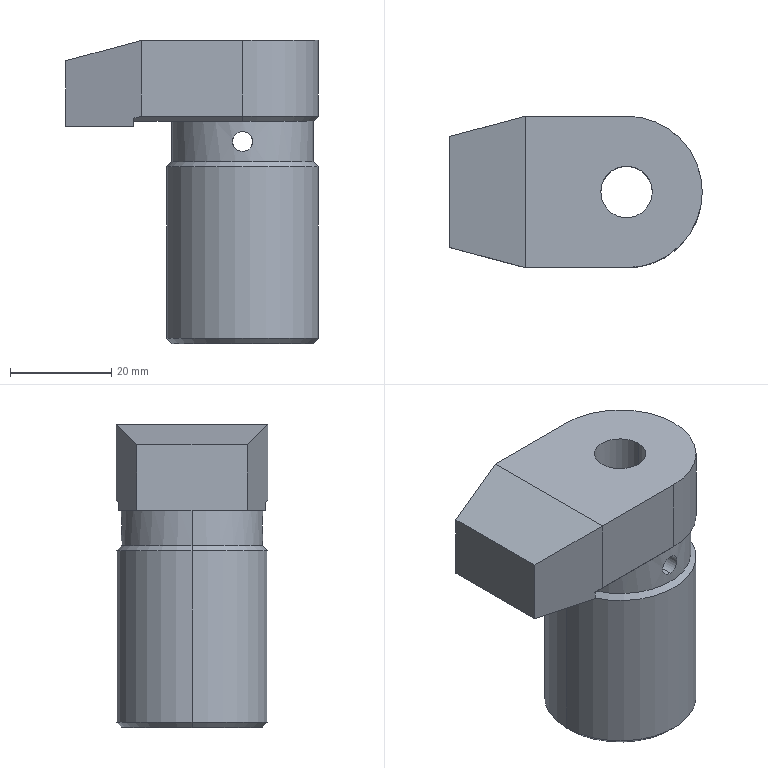Part | SolidWorks | features ICE 7, Chamfer 2, 3DProfileFeature 1, Extrusion 1, HoleWzd 1, MirrorPattern 1 | 1 solid | 36 faces | box 50 x 30 x 60 mm | volume 40900 mm3 | cylinder 15 | plane 13 | cone 8 | commonest cylinder face diameters 4 x4 30 x4 10.2 x2 18 x2 28 x2 52 x1
STEP:
#1=CARTESIAN_POINT('',(0.,14.,-22.));
#2=VERTEX_POINT('',#1);
#3=CARTESIAN_POINT('',(0.,14.,-18.));
#4=VERTEX_POINT('',#3);
#5=CARTESIAN_POINT('',(0.,14.,-22.));
#6=CARTESIAN_POINT('',(-0.1323,14.,-22.));
#7=CARTESIAN_POINT('',(-0.2624,13.998,-21.987));
#8=CARTESIAN_POINT('',(-0.5183,13.991,-21.936));
#9=CARTESIAN_POINT('',(-0.6454,13.986,-21.898));
#10=CARTESIAN_POINT('',(-0.8875,13.972,-21.797));
#11=CARTESIAN_POINT('',(-1.002,13.964,-21.736));
#12=CARTESIAN_POINT('',(-1.22,13.947,-21.59));
#13=CARTESIAN_POINT('',(-1.322,13.938,-21.506));
#14=CARTESIAN_POINT('',(-1.599,13.91,-21.23));
#15=CARTESIAN_POINT('',(-1.748,13.891,-21.007));
#16=CARTESIAN_POINT('',(-1.947,13.864,-20.525));
#17=CARTESIAN_POINT('',(-2.,13.856,-20.262));
#18=CARTESIAN_POINT('',(-2.,13.856,-19.87));
#19=CARTESIAN_POINT('',(-1.987,13.858,-19.737));
#20=CARTESIAN_POINT('',(-1.936,13.866,-19.481));
#21=CARTESIAN_POINT('',(-1.898,13.871,-19.356));
#22=CARTESIAN_POINT('',(-1.798,13.884,-19.114));
#23=CARTESIAN_POINT('',(-1.735,13.892,-18.997));
#24=CARTESIAN_POINT('',(-1.59,13.91,-18.78));
#25=CARTESIAN_POINT('',(-1.508,13.919,-18.679));
#26=CARTESIAN_POINT('',(-1.321,13.938,-18.493));
#27=CARTESIAN_POINT('',(-1.22,13.947,-18.41));
#28=CARTESIAN_POINT('',(-1.004,13.964,-18.265));
#29=CARTESIAN_POINT('',(-0.8867,13.972,-18.203));
#30=CARTESIAN_POINT('',(-0.6447,13.986,-18.102));
#31=CARTESIAN_POINT('',(-0.52,13.991,-18.064));
#32=CARTESIAN_POINT('',(-0.2633,13.998,-18.013));
#33=CARTESIAN_POINT('',(-0.1306,14.,-18.));
#34=CARTESIAN_POINT('',(0.,14.,-18.));
#35=B_SPLINE_CURVE_WITH_KNOTS('',3,(#5,#6,#7,#8,#9,#10,#11,#12,#13,#14,#15,#16,#17,#18,#19,#20,#21,#22,#23,#24,#25,#26,#27,#28,#29,#30,#31,#32,#33,#34),.UNSPECIFIED.,.F.,.F.,(4,2,2,2,2,2,2,2,2,2,2,2,2,2,4),(0.,0.0003913,0.0007826,0.001174,0.001565,0.002348,0.00313,0.003522,0.003913,0.004304,0.004696,0.005087,0.005478,0.00587,0.006261),.UNSPECIFIED.);
#36=EDGE_CURVE('',#2,#4,#35,.T.);
#37=ORIENTED_EDGE('',*,*,#36,.T.);
#38=CARTESIAN_POINT('',(0.,5.1,-18.));
#39=VERTEX_POINT('',#38);
#40=CARTESIAN_POINT('',(0.,30.,-18.));
#41=DIRECTION('',(0.,-1.,0.));
#42=VECTOR('',#41,1000.);
#43=LINE('',#40,#42);
#44=EDGE_CURVE('',#4,#39,#43,.T.);
#45=ORIENTED_EDGE('',*,*,#44,.T.);
#46=CARTESIAN_POINT('',(0.,5.1,-22.));
#47=VERTEX_POINT('',#46);
#48=CARTESIAN_POINT('',(0.,5.1,-18.));
#49=CARTESIAN_POINT('',(-0.1316,5.1,-18.));
#50=CARTESIAN_POINT('',(-0.2648,5.095,-18.013));
#51=CARTESIAN_POINT('',(-0.5241,5.075,-18.065));
#52=CARTESIAN_POINT('',(-0.6493,5.06,-18.104));
#53=CARTESIAN_POINT('',(-0.8913,5.023,-18.205));
#54=CARTESIAN_POINT('',(-1.008,5.001,-18.268));
#55=CARTESIAN_POINT('',(-1.223,4.952,-18.412));
#56=CARTESIAN_POINT('',(-1.323,4.926,-18.495));
#57=CARTESIAN_POINT('',(-1.508,4.873,-18.68));
#58=CARTESIAN_POINT('',(-1.59,4.846,-18.78));
#59=CARTESIAN_POINT('',(-1.734,4.797,-18.995));
#60=CARTESIAN_POINT('',(-1.796,4.773,-19.111));
#61=CARTESIAN_POINT('',(-1.897,4.734,-19.353));
#62=CARTESIAN_POINT('',(-1.935,4.719,-19.478));
#63=CARTESIAN_POINT('',(-1.987,4.697,-19.735));
#64=CARTESIAN_POINT('',(-2.,4.691,-19.869));
#65=CARTESIAN_POINT('',(-2.,4.692,-20.265));
#66=CARTESIAN_POINT('',(-1.946,4.715,-20.53));
#67=CARTESIAN_POINT('',(-1.795,4.774,-20.891));
#68=CARTESIAN_POINT('',(-1.732,4.797,-21.008));
#69=CARTESIAN_POINT('',(-1.587,4.847,-21.224));
#70=CARTESIAN_POINT('',(-1.505,4.874,-21.323));
#71=CARTESIAN_POINT('',(-1.322,4.927,-21.507));
#72=CARTESIAN_POINT('',(-1.22,4.953,-21.59));
#73=CARTESIAN_POINT('',(-1.005,5.001,-21.734));
#74=CARTESIAN_POINT('',(-0.8903,5.023,-21.796));
#75=CARTESIAN_POINT('',(-0.5249,5.079,-21.948));
#76=CARTESIAN_POINT('',(-0.2671,5.1,-22.));
#77=CARTESIAN_POINT('',(0.,5.1,-22.));
#78=B_SPLINE_CURVE_WITH_KNOTS('',3,(#48,#49,#50,#51,#52,#53,#54,#55,#56,#57,#58,#59,#60,#61,#62,#63,#64,#65,#66,#67,#68,#69,#70,#71,#72,#73,#74,#75,#76,#77),.UNSPECIFIED.,.F.,.F.,(4,2,2,2,2,2,2,2,2,2,2,2,2,2,4),(0.006317,0.006712,0.007106,0.007501,0.007896,0.008291,0.008685,0.00908,0.009475,0.01026,0.01066,0.01105,0.01145,0.01184,0.01263),.UNSPECIFIED.);
#79=EDGE_CURVE('',#39,#47,#78,.T.);
#80=ORIENTED_EDGE('',*,*,#79,.T.);
#81=CARTESIAN_POINT('',(0.,30.,-22.));
#82=DIRECTION('',(0.,-1.,0.));
#83=VECTOR('',#82,1000.);
#84=LINE('',#81,#83);
#85=EDGE_CURVE('',#2,#47,#84,.T.);
#86=ORIENTED_EDGE('',*,*,#85,.F.);
#87=EDGE_LOOP('',(#37,#45,#80,#86));
#88=FACE_OUTER_BOUND('',#87,.T.);
#89=CARTESIAN_POINT('',(0.,30.,-20.));
#90=DIRECTION('',(0.,-1.,0.));
#91=DIRECTION('',(0.,0.,-1.));
#92=AXIS2_PLACEMENT_3D('',#89,#90,#91);
#93=CYLINDRICAL_SURFACE('',#92,2.);
#94=ADVANCED_FACE('',(#88),#93,.F.);
#95=CARTESIAN_POINT('',(0.,-5.1,-22.));
#96=VERTEX_POINT('',#95);
#97=CARTESIAN_POINT('',(0.,-5.1,-18.));
#98=VERTEX_POINT('',#97);
#99=CARTESIAN_POINT('',(0.,-5.1,-22.));
#100=CARTESIAN_POINT('',(-0.1336,-5.1,-22.));
#101=CARTESIAN_POINT('',(-0.2647,-5.095,-21.987));
#102=CARTESIAN_POINT('',(-0.5222,-5.075,-21.935));
#103=CARTESIAN_POINT('',(-0.65,-5.06,-21.896));
#104=CARTESIAN_POINT('',(-0.8917,-5.023,-21.795));
#105=CARTESIAN_POINT('',(-1.006,-5.001,-21.733));
#106=CARTESIAN_POINT('',(-1.223,-4.953,-21.588));
#107=CARTESIAN_POINT('',(-1.324,-4.926,-21.505));
#108=CARTESIAN_POINT('',(-1.598,-4.847,-21.231));
#109=CARTESIAN_POINT('',(-1.746,-4.793,-21.01));
#110=CARTESIAN_POINT('',(-1.896,-4.735,-20.65));
#111=CARTESIAN_POINT('',(-1.935,-4.719,-20.523));
#112=CARTESIAN_POINT('',(-1.987,-4.697,-20.264));
#113=CARTESIAN_POINT('',(-2.,-4.692,-20.133));
#114=CARTESIAN_POINT('',(-2.,-4.691,-19.869));
#115=CARTESIAN_POINT('',(-1.987,-4.697,-19.735));
#116=CARTESIAN_POINT('',(-1.935,-4.719,-19.477));
#117=CARTESIAN_POINT('',(-1.897,-4.734,-19.352));
#118=CARTESIAN_POINT('',(-1.795,-4.774,-19.108));
#119=CARTESIAN_POINT('',(-1.733,-4.797,-18.994));
#120=CARTESIAN_POINT('',(-1.589,-4.847,-18.778));
#121=CARTESIAN_POINT('',(-1.505,-4.874,-18.677));
#122=CARTESIAN_POINT('',(-1.322,-4.927,-18.494));
#123=CARTESIAN_POINT('',(-1.222,-4.953,-18.412));
#124=CARTESIAN_POINT('',(-1.006,-5.001,-18.267));
#125=CARTESIAN_POINT('',(-0.8896,-5.023,-18.204));
#126=CARTESIAN_POINT('',(-0.5289,-5.078,-18.054));
#127=CARTESIAN_POINT('',(-0.2632,-5.1,-18.));
#128=CARTESIAN_POINT('',(0.,-5.1,-18.));
#129=B_SPLINE_CURVE_WITH_KNOTS('',3,(#99,#100,#101,#102,#103,#104,#105,#106,#107,#108,#109,#110,#111,#112,#113,#114,#115,#116,#117,#118,#119,#120,#121,#122,#123,#124,#125,#126,#127,#128),.UNSPECIFIED.,.F.,.F.,(4,2,2,2,2,2,2,2,2,2,2,2,2,2,4),(0.,0.0003948,0.0007896,0.001184,0.001579,0.002369,0.002764,0.003158,0.003553,0.003948,0.004343,0.004738,0.005133,0.005527,0.006317),.UNSPECIFIED.);
#130=EDGE_CURVE('',#96,#98,#129,.T.);
#131=ORIENTED_EDGE('',*,*,#130,.T.);
#132=CARTESIAN_POINT('',(0.,-14.,-18.));
#133=VERTEX_POINT('',#132);
#134=CARTESIAN_POINT('',(0.,30.,-18.));
#135=DIRECTION('',(0.,-1.,0.));
#136=VECTOR('',#135,1000.);
#137=LINE('',#134,#136);
#138=EDGE_CURVE('',#98,#133,#137,.T.);
#139=ORIENTED_EDGE('',*,*,#138,.T.);
#140=CARTESIAN_POINT('',(0.,-14.,-22.));
#141=VERTEX_POINT('',#140);
#142=CARTESIAN_POINT('',(0.,-14.,-18.));
#143=CARTESIAN_POINT('',(-0.2612,-14.,-18.));
#144=CARTESIAN_POINT('',(-0.5246,-13.992,-18.053));
#145=CARTESIAN_POINT('',(-1.006,-13.966,-18.252));
#146=CARTESIAN_POINT('',(-1.229,-13.947,-18.401));
#147=CARTESIAN_POINT('',(-1.506,-13.919,-18.677));
#148=CARTESIAN_POINT('',(-1.59,-13.91,-18.78));
#149=CARTESIAN_POINT('',(-1.735,-13.892,-18.997));
#150=CARTESIAN_POINT('',(-1.797,-13.884,-19.111));
#151=CARTESIAN_POINT('',(-1.897,-13.871,-19.354));
#152=CARTESIAN_POINT('',(-1.936,-13.866,-19.481));
#153=CARTESIAN_POINT('',(-1.987,-13.858,-19.736));
#154=CARTESIAN_POINT('',(-2.,-13.856,-19.866));
#155=CARTESIAN_POINT('',(-2.,-13.856,-20.131));
#156=CARTESIAN_POINT('',(-1.987,-13.858,-20.261));
#157=CARTESIAN_POINT('',(-1.936,-13.865,-20.517));
#158=CARTESIAN_POINT('',(-1.898,-13.871,-20.644));
#159=CARTESIAN_POINT('',(-1.798,-13.884,-20.886));
#160=CARTESIAN_POINT('',(-1.736,-13.892,-21.001));
#161=CARTESIAN_POINT('',(-1.591,-13.909,-21.218));
#162=CARTESIAN_POINT('',(-1.507,-13.919,-21.321));
#163=CARTESIAN_POINT('',(-1.231,-13.947,-21.598));
#164=CARTESIAN_POINT('',(-1.008,-13.966,-21.747));
#165=CARTESIAN_POINT('',(-0.5274,-13.992,-21.947));
#166=CARTESIAN_POINT('',(-0.2646,-14.,-22.));
#167=CARTESIAN_POINT('',(0.,-14.,-22.));
#168=B_SPLINE_CURVE_WITH_KNOTS('',3,(#142,#143,#144,#145,#146,#147,#148,#149,#150,#151,#152,#153,#154,#155,#156,#157,#158,#159,#160,#161,#162,#163,#164,#165,#166,#167),.UNSPECIFIED.,.F.,.F.,(4,2,2,2,2,2,2,2,2,2,2,2,4),(0.006261,0.007043,0.007826,0.008217,0.008608,0.008999,0.009391,0.009782,0.01017,0.01056,0.01096,0.01174,0.01252),.UNSPECIFIED.);
#169=EDGE_CURVE('',#133,#141,#168,.T.);
#170=ORIENTED_EDGE('',*,*,#169,.T.);
#171=CARTESIAN_POINT('',(0.,30.,-22.));
#172=DIRECTION('',(0.,-1.,0.));
#173=VECTOR('',#172,1000.);
#174=LINE('',#171,#173);
#175=EDGE_CURVE('',#96,#141,#174,.T.);
#176=ORIENTED_EDGE('',*,*,#175,.F.);
#177=EDGE_LOOP('',(#131,#139,#170,#176));
#178=FACE_OUTER_BOUND('',#177,.T.);
#179=CARTESIAN_POINT('',(0.,30.,-20.));
#180=DIRECTION('',(0.,-1.,0.));
#181=DIRECTION('',(0.,0.,-1.));
#182=AXIS2_PLACEMENT_3D('',#179,#180,#181);
#183=CYLINDRICAL_SURFACE('',#182,2.);
#184=ADVANCED_FACE('',(#178),#183,.F.);
#185=CARTESIAN_POINT('',(9.,0.,-59.));
#186=VERTEX_POINT('',#185);
#187=CARTESIAN_POINT('',(-9.,0.,-59.));
#188=VERTEX_POINT('',#187);
#189=CARTESIAN_POINT('',(0.,0.,-59.));
#190=DIRECTION('',(0.,0.,-1.));
#191=DIRECTION('',(-1.,0.,0.));
#192=AXIS2_PLACEMENT_3D('',#189,#190,#191);
#193=CIRCLE('',#192,9.);
#194=EDGE_CURVE('',#186,#188,#193,.T.);
#195=ORIENTED_EDGE('',*,*,#194,.F.);
#196=CARTESIAN_POINT('',(10.,0.,-60.));
#197=VERTEX_POINT('',#196);
#198=CARTESIAN_POINT('',(9.,0.,-59.));
#199=DIRECTION('',(0.7071,0.,-0.7071));
#200=VECTOR('',#199,1000.);
#201=LINE('',#198,#200);
#202=EDGE_CURVE('',#186,#197,#201,.T.);
#203=ORIENTED_EDGE('',*,*,#202,.T.);
#204=CARTESIAN_POINT('',(-10.,0.,-60.));
#205=VERTEX_POINT('',#204);
#206=CARTESIAN_POINT('',(0.,0.,-60.));
#207=DIRECTION('',(0.,0.,1.));
#208=DIRECTION('',(-1.,0.,0.));
#209=AXIS2_PLACEMENT_3D('',#206,#207,#208);
#210=CIRCLE('',#209,10.);
#211=EDGE_CURVE('',#205,#197,#210,.T.);
#212=ORIENTED_EDGE('',*,*,#211,.F.);
#213=CARTESIAN_POINT('',(-9.,0.,-59.));
#214=DIRECTION('',(-0.7071,0.,-0.7071));
#215=VECTOR('',#214,1000.);
#216=LINE('',#213,#215);
#217=EDGE_CURVE('',#188,#205,#216,.T.);
#218=ORIENTED_EDGE('',*,*,#217,.F.);
#219=EDGE_LOOP('',(#195,#203,#212,#218));
#220=FACE_OUTER_BOUND('',#219,.T.);
#221=CARTESIAN_POINT('',(0.,0.,-59.));
#222=DIRECTION('',(0.,0.,-1.));
#223=DIRECTION('',(-1.,0.,0.));
#224=AXIS2_PLACEMENT_3D('',#221,#222,#223);
#225=CONICAL_SURFACE('',#224,9.,0.7854);
#226=ADVANCED_FACE('',(#220),#225,.F.);
#227=CARTESIAN_POINT('',(-14.,0.,-60.));
#228=VERTEX_POINT('',#227);
#229=CARTESIAN_POINT('',(14.,0.,-60.));
#230=VERTEX_POINT('',#229);
#231=CARTESIAN_POINT('',(0.,0.,-60.));
#232=DIRECTION('',(0.,0.,-1.));
#233=DIRECTION('',(-1.,0.,0.));
#234=AXIS2_PLACEMENT_3D('',#231,#232,#233);
#235=CIRCLE('',#234,14.);
#236=EDGE_CURVE('',#228,#230,#235,.T.);
#237=ORIENTED_EDGE('',*,*,#236,.F.);
#238=CARTESIAN_POINT('',(-15.,0.,-59.));
#239=VERTEX_POINT('',#238);
#240=CARTESIAN_POINT('',(-14.,0.,-60.));
#241=DIRECTION('',(-0.7071,0.,0.7071));
#242=VECTOR('',#241,1000.);
#243=LINE('',#240,#242);
#244=EDGE_CURVE('',#228,#239,#243,.T.);
#245=ORIENTED_EDGE('',*,*,#244,.T.);
#246=CARTESIAN_POINT('',(15.,0.,-59.));
#247=VERTEX_POINT('',#246);
#248=CARTESIAN_POINT('',(0.,0.,-59.));
#249=DIRECTION('',(0.,0.,1.));
#250=DIRECTION('',(-1.,0.,0.));
#251=AXIS2_PLACEMENT_3D('',#248,#249,#250);
#252=CIRCLE('',#251,15.);
#253=EDGE_CURVE('',#247,#239,#252,.T.);
#254=ORIENTED_EDGE('',*,*,#253,.F.);
#255=CARTESIAN_POINT('',(14.,0.,-60.));
#256=DIRECTION('',(0.7071,0.,0.7071));
#257=VECTOR('',#256,1000.);
#258=LINE('',#255,#257);
#259=EDGE_CURVE('',#230,#247,#258,.T.);
#260=ORIENTED_EDGE('',*,*,#259,.F.);
#261=EDGE_LOOP('',(#237,#245,#254,#260));
#262=FACE_OUTER_BOUND('',#261,.T.);
#263=CARTESIAN_POINT('',(0.,0.,-60.));
#264=DIRECTION('',(0.,0.,1.));
#265=DIRECTION('',(1.,0.,0.));
#266=AXIS2_PLACEMENT_3D('',#263,#264,#265);
#267=CONICAL_SURFACE('',#266,14.,0.7854);
#268=ADVANCED_FACE('',(#262),#267,.T.);
#269=CARTESIAN_POINT('',(9.,0.,-30.));
#270=VERTEX_POINT('',#269);
#271=CARTESIAN_POINT('',(-9.,0.,-30.));
#272=VERTEX_POINT('',#271);
#273=CARTESIAN_POINT('',(0.,0.,-30.));
#274=DIRECTION('',(0.,0.,-1.));
#275=DIRECTION('',(-1.,0.,0.));
#276=AXIS2_PLACEMENT_3D('',#273,#274,#275);
#277=CIRCLE('',#276,9.);
#278=EDGE_CURVE('',#270,#272,#277,.T.);
#279=ORIENTED_EDGE('',*,*,#278,.F.);
#280=CARTESIAN_POINT('',(9.,0.,-30.));
#281=DIRECTION('',(0.,0.,-1.));
#282=VECTOR('',#281,1000.);
#283=LINE('',#280,#282);
#284=EDGE_CURVE('',#270,#186,#283,.T.);
#285=ORIENTED_EDGE('',*,*,#284,.T.);
#286=ORIENTED_EDGE('',*,*,#194,.T.);
#287=CARTESIAN_POINT('',(-9.,0.,-30.));
#288=DIRECTION('',(0.,0.,-1.));
#289=VECTOR('',#288,1000.);
#290=LINE('',#287,#289);
#291=EDGE_CURVE('',#272,#188,#290,.T.);
#292=ORIENTED_EDGE('',*,*,#291,.F.);
#293=EDGE_LOOP('',(#279,#285,#286,#292));
#294=FACE_OUTER_BOUND('',#293,.T.);
#295=CARTESIAN_POINT('',(0.,0.,-30.));
#296=DIRECTION('',(0.,0.,-1.));
#297=DIRECTION('',(-1.,0.,0.));
#298=AXIS2_PLACEMENT_3D('',#295,#296,#297);
#299=CYLINDRICAL_SURFACE('',#298,9.);
#300=ADVANCED_FACE('',(#294),#299,.F.);
#301=CARTESIAN_POINT('',(14.,0.,-16.));
#302=VERTEX_POINT('',#301);
#303=CARTESIAN_POINT('',(0.,-14.,-16.));
#304=VERTEX_POINT('',#303);
#305=CARTESIAN_POINT('',(0.,0.,-16.));
#306=DIRECTION('',(0.,0.,-1.));
#307=DIRECTION('',(-1.,0.,0.));
#308=AXIS2_PLACEMENT_3D('',#305,#306,#307);
#309=CIRCLE('',#308,14.);
#310=EDGE_CURVE('',#302,#304,#309,.T.);
#311=ORIENTED_EDGE('',*,*,#310,.F.);
#312=CARTESIAN_POINT('',(15.,0.,-15.));
#313=VERTEX_POINT('',#312);
#314=CARTESIAN_POINT('',(14.,0.,-16.));
#315=DIRECTION('',(0.7071,0.,0.7071));
#316=VECTOR('',#315,1000.);
#317=LINE('',#314,#316);
#318=EDGE_CURVE('',#302,#313,#317,.T.);
#319=ORIENTED_EDGE('',*,*,#318,.T.);
#320=CARTESIAN_POINT('',(0.,-15.,-15.));
#321=VERTEX_POINT('',#320);
#322=CARTESIAN_POINT('',(0.,0.,-15.));
#323=DIRECTION('',(0.,0.,1.));
#324=DIRECTION('',(1.,0.,0.));
#325=AXIS2_PLACEMENT_3D('',#322,#323,#324);
#326=CIRCLE('',#325,15.);
#327=EDGE_CURVE('',#321,#313,#326,.T.);
#328=ORIENTED_EDGE('',*,*,#327,.F.);
#329=CARTESIAN_POINT('',(0.,-15.,-15.));
#330=DIRECTION('',(0.,0.7071,-0.7071));
#331=VECTOR('',#330,1000.);
#332=LINE('',#329,#331);
#333=EDGE_CURVE('',#321,#304,#332,.T.);
#334=ORIENTED_EDGE('',*,*,#333,.T.);
#335=EDGE_LOOP('',(#311,#319,#328,#334));
#336=FACE_OUTER_BOUND('',#335,.T.);
#337=CARTESIAN_POINT('',(0.,0.,-16.));
#338=DIRECTION('',(0.,0.,1.));
#339=DIRECTION('',(1.,0.,0.));
#340=AXIS2_PLACEMENT_3D('',#337,#338,#339);
#341=CONICAL_SURFACE('',#340,14.,0.7854);
#342=ADVANCED_FACE('',(#336),#341,.T.);
#343=CARTESIAN_POINT('',(-14.,0.,-24.));
#344=VERTEX_POINT('',#343);
#345=CARTESIAN_POINT('',(14.,0.,-24.));
#346=VERTEX_POINT('',#345);
#347=CARTESIAN_POINT('',(0.,0.,-24.));
#348=DIRECTION('',(0.,0.,-1.));
#349=DIRECTION('',(-1.,0.,0.));
#350=AXIS2_PLACEMENT_3D('',#347,#348,#349);
#351=CIRCLE('',#350,14.);
#352=EDGE_CURVE('',#344,#346,#351,.T.);
#353=ORIENTED_EDGE('',*,*,#352,.T.);
#354=CARTESIAN_POINT('',(15.,0.,-25.));
#355=VERTEX_POINT('',#354);
#356=CARTESIAN_POINT('',(15.,0.,-25.));
#357=DIRECTION('',(0.7071,0.,-0.7071));
#358=VECTOR('',#357,1000.);
#359=LINE('',#356,#358);
#360=EDGE_CURVE('',#346,#355,#359,.T.);
#361=ORIENTED_EDGE('',*,*,#360,.T.);
#362=CARTESIAN_POINT('',(-15.,0.,-25.));
#363=VERTEX_POINT('',#362);
#364=CARTESIAN_POINT('',(0.,0.,-25.));
#365=DIRECTION('',(0.,0.,-1.));
#366=DIRECTION('',(-1.,0.,0.));
#367=AXIS2_PLACEMENT_3D('',#364,#365,#366);
#368=CIRCLE('',#367,15.);
#369=EDGE_CURVE('',#363,#355,#368,.T.);
#370=ORIENTED_EDGE('',*,*,#369,.F.);
#371=CARTESIAN_POINT('',(-15.,0.,-25.));
#372=DIRECTION('',(-0.7071,0.,-0.7071));
#373=VECTOR('',#372,1000.);
#374=LINE('',#371,#373);
#375=EDGE_CURVE('',#344,#363,#374,.T.);
#376=ORIENTED_EDGE('',*,*,#375,.F.);
#377=EDGE_LOOP('',(#353,#361,#370,#376));
#378=FACE_OUTER_BOUND('',#377,.T.);
#379=CARTESIAN_POINT('',(0.,0.,-25.));
#380=DIRECTION('',(0.,0.,-1.));
#381=DIRECTION('',(-1.,0.,0.));
#382=AXIS2_PLACEMENT_3D('',#379,#380,#381);
#383=CONICAL_SURFACE('',#382,15.,0.7854);
#384=ADVANCED_FACE('',(#378),#383,.T.);
#385=ORIENTED_EDGE('',*,*,#253,.T.);
#386=CARTESIAN_POINT('',(-15.,0.,-16.));
#387=DIRECTION('',(0.,0.,1.));
#388=VECTOR('',#387,1000.);
#389=LINE('',#386,#388);
#390=EDGE_CURVE('',#239,#363,#389,.T.);
#391=ORIENTED_EDGE('',*,*,#390,.T.);
#392=ORIENTED_EDGE('',*,*,#369,.T.);
#393=CARTESIAN_POINT('',(15.,0.,-16.));
#394=DIRECTION('',(0.,0.,1.));
#395=VECTOR('',#394,1000.);
#396=LINE('',#393,#395);
#397=EDGE_CURVE('',#247,#355,#396,.T.);
#398=ORIENTED_EDGE('',*,*,#397,.F.);
#399=EDGE_LOOP('',(#385,#391,#392,#398));
#400=FACE_OUTER_BOUND('',#399,.T.);
#401=CARTESIAN_POINT('',(0.,0.,-16.));
#402=DIRECTION('',(0.,0.,1.));
#403=DIRECTION('',(1.,0.,0.));
#404=AXIS2_PLACEMENT_3D('',#401,#402,#403);
#405=CYLINDRICAL_SURFACE('',#404,15.);
#406=ADVANCED_FACE('',(#400),#405,.T.);
#407=ORIENTED_EDGE('',*,*,#327,.T.);
#408=CARTESIAN_POINT('',(15.,0.,0.));
#409=VERTEX_POINT('',#408);
#410=CARTESIAN_POINT('',(15.,0.,-16.));
#411=DIRECTION('',(0.,0.,1.));
#412=VECTOR('',#411,1000.);
#413=LINE('',#410,#412);
#414=EDGE_CURVE('',#313,#409,#413,.T.);
#415=ORIENTED_EDGE('',*,*,#414,.T.);
#416=CARTESIAN_POINT('',(0.,-15.,0.));
#417=VERTEX_POINT('',#416);
#418=CARTESIAN_POINT('',(0.,0.,0.));
#419=DIRECTION('',(0.,0.,1.));
#420=DIRECTION('',(1.,0.,0.));
#421=AXIS2_PLACEMENT_3D('',#418,#419,#420);
#422=CIRCLE('',#421,15.);
#423=EDGE_CURVE('',#417,#409,#422,.T.);
#424=ORIENTED_EDGE('',*,*,#423,.F.);
#425=CARTESIAN_POINT('',(0.,-15.,-16.));
#426=DIRECTION('',(0.,0.,1.));
#427=VECTOR('',#426,1000.);
#428=LINE('',#425,#427);
#429=EDGE_CURVE('',#321,#417,#428,.T.);
#430=ORIENTED_EDGE('',*,*,#429,.F.);
#431=EDGE_LOOP('',(#407,#415,#424,#430));
#432=FACE_OUTER_BOUND('',#431,.T.);
#433=CARTESIAN_POINT('',(0.,0.,-16.));
#434=DIRECTION('',(0.,0.,1.));
#435=DIRECTION('',(1.,0.,0.));
#436=AXIS2_PLACEMENT_3D('',#433,#434,#435);
#437=CYLINDRICAL_SURFACE('',#436,15.);
#438=ADVANCED_FACE('',(#432),#437,.T.);
#439=ORIENTED_EDGE('',*,*,#130,.F.);
#440=CARTESIAN_POINT('',(0.,-5.1,-18.));
#441=CARTESIAN_POINT('',(0.1316,-5.1,-18.));
#442=CARTESIAN_POINT('',(0.2648,-5.095,-18.013));
#443=CARTESIAN_POINT('',(0.5241,-5.075,-18.065));
#444=CARTESIAN_POINT('',(0.6493,-5.06,-18.104));
#445=CARTESIAN_POINT('',(0.8913,-5.023,-18.205));
#446=CARTESIAN_POINT('',(1.008,-5.001,-18.268));
#447=CARTESIAN_POINT('',(1.223,-4.952,-18.412));
#448=CARTESIAN_POINT('',(1.323,-4.926,-18.495));
#449=CARTESIAN_POINT('',(1.508,-4.873,-18.68));
#450=CARTESIAN_POINT('',(1.59,-4.846,-18.78));
#451=CARTESIAN_POINT('',(1.734,-4.797,-18.995));
#452=CARTESIAN_POINT('',(1.796,-4.773,-19.111));
#453=CARTESIAN_POINT('',(1.897,-4.734,-19.353));
#454=CARTESIAN_POINT('',(1.935,-4.719,-19.478));
#455=CARTESIAN_POINT('',(1.987,-4.697,-19.735));
#456=CARTESIAN_POINT('',(2.,-4.691,-19.869));
#457=CARTESIAN_POINT('',(2.,-4.692,-20.265));
#458=CARTESIAN_POINT('',(1.946,-4.715,-20.53));
#459=CARTESIAN_POINT('',(1.795,-4.774,-20.891));
#460=CARTESIAN_POINT('',(1.732,-4.797,-21.008));
#461=CARTESIAN_POINT('',(1.587,-4.847,-21.224));
#462=CARTESIAN_POINT('',(1.505,-4.874,-21.323));
#463=CARTESIAN_POINT('',(1.322,-4.927,-21.507));
#464=CARTESIAN_POINT('',(1.22,-4.953,-21.59));
#465=CARTESIAN_POINT('',(1.005,-5.001,-21.734));
#466=CARTESIAN_POINT('',(0.8903,-5.023,-21.796));
#467=CARTESIAN_POINT('',(0.5249,-5.079,-21.948));
#468=CARTESIAN_POINT('',(0.2671,-5.1,-22.));
#469=CARTESIAN_POINT('',(0.,-5.1,-22.));
#470=B_SPLINE_CURVE_WITH_KNOTS('',3,(#440,#441,#442,#443,#444,#445,#446,#447,#448,#449,#450,#451,#452,#453,#454,#455,#456,#457,#458,#459,#460,#461,#462,#463,#464,#465,#466,#467,#468,#469),.UNSPECIFIED.,.F.,.F.,(4,2,2,2,2,2,2,2,2,2,2,2,2,2,4),(0.006317,0.006712,0.007106,0.007501,0.007896,0.008291,0.008685,0.00908,0.009475,0.01026,0.01066,0.01105,0.01145,0.01184,0.01263),.UNSPECIFIED.);
#471=EDGE_CURVE('',#98,#96,#470,.T.);
#472=ORIENTED_EDGE('',*,*,#471,.F.);
#473=EDGE_LOOP('',(#439,#472));
#474=FACE_BOUND('',#473,.T.);
#475=CARTESIAN_POINT('',(5.1,0.,-30.));
#476=VERTEX_POINT('',#475);
#477=CARTESIAN_POINT('',(-5.1,0.,-30.));
#478=VERTEX_POINT('',#477);
#479=CARTESIAN_POINT('',(0.,0.,-30.));
#480=DIRECTION('',(0.,0.,-1.));
#481=DIRECTION('',(-1.,0.,0.));
#482=AXIS2_PLACEMENT_3D('',#479,#480,#481);
#483=CIRCLE('',#482,5.1);
#484=EDGE_CURVE('',#476,#478,#483,.T.);
#485=ORIENTED_EDGE('',*,*,#484,.T.);
#486=CARTESIAN_POINT('',(-5.1,0.,0.));
#487=VERTEX_POINT('',#486);
#488=CARTESIAN_POINT('',(-5.1,0.,0.));
#489=DIRECTION('',(0.,0.,1.));
#490=VECTOR('',#489,1000.);
#491=LINE('',#488,#490);
#492=EDGE_CURVE('',#478,#487,#491,.T.);
#493=ORIENTED_EDGE('',*,*,#492,.T.);
#494=CARTESIAN_POINT('',(5.1,0.,0.));
#495=VERTEX_POINT('',#494);
#496=CARTESIAN_POINT('',(0.,0.,0.));
#497=DIRECTION('',(0.,0.,1.));
#498=DIRECTION('',(1.,0.,0.));
#499=AXIS2_PLACEMENT_3D('',#496,#497,#498);
#500=CIRCLE('',#499,5.1);
#501=EDGE_CURVE('',#487,#495,#500,.T.);
#502=ORIENTED_EDGE('',*,*,#501,.T.);
#503=CARTESIAN_POINT('',(5.1,0.,0.));
#504=DIRECTION('',(0.,0.,1.));
#505=VECTOR('',#504,1000.);
#506=LINE('',#503,#505);
#507=EDGE_CURVE('',#476,#495,#506,.T.);
#508=ORIENTED_EDGE('',*,*,#507,.F.);
#509=EDGE_LOOP('',(#485,#493,#502,#508));
#510=FACE_OUTER_BOUND('',#509,.T.);
#511=CARTESIAN_POINT('',(0.,0.,0.));
#512=DIRECTION('',(0.,0.,1.));
#513=DIRECTION('',(1.,0.,0.));
#514=AXIS2_PLACEMENT_3D('',#511,#512,#513);
#515=CYLINDRICAL_SURFACE('',#514,5.1);
#516=ADVANCED_FACE('',(#474,#510),#515,.F.);
#517=ORIENTED_EDGE('',*,*,#36,.F.);
#518=CARTESIAN_POINT('',(0.,14.,-18.));
#519=CARTESIAN_POINT('',(0.2612,14.,-18.));
#520=CARTESIAN_POINT('',(0.5246,13.992,-18.053));
#521=CARTESIAN_POINT('',(1.006,13.966,-18.252));
#522=CARTESIAN_POINT('',(1.229,13.947,-18.401));
#523=CARTESIAN_POINT('',(1.506,13.919,-18.677));
#524=CARTESIAN_POINT('',(1.59,13.91,-18.78));
#525=CARTESIAN_POINT('',(1.735,13.892,-18.997));
#526=CARTESIAN_POINT('',(1.797,13.884,-19.111));
#527=CARTESIAN_POINT('',(1.897,13.871,-19.354));
#528=CARTESIAN_POINT('',(1.936,13.866,-19.481));
#529=CARTESIAN_POINT('',(1.987,13.858,-19.736));
#530=CARTESIAN_POINT('',(2.,13.856,-19.866));
#531=CARTESIAN_POINT('',(2.,13.856,-20.131));
#532=CARTESIAN_POINT('',(1.987,13.858,-20.261));
#533=CARTESIAN_POINT('',(1.936,13.865,-20.517));
#534=CARTESIAN_POINT('',(1.898,13.871,-20.644));
#535=CARTESIAN_POINT('',(1.798,13.884,-20.886));
#536=CARTESIAN_POINT('',(1.736,13.892,-21.001));
#537=CARTESIAN_POINT('',(1.591,13.909,-21.218));
#538=CARTESIAN_POINT('',(1.507,13.919,-21.321));
#539=CARTESIAN_POINT('',(1.231,13.947,-21.598));
#540=CARTESIAN_POINT('',(1.008,13.966,-21.747));
#541=CARTESIAN_POINT('',(0.5274,13.992,-21.947));
#542=CARTESIAN_POINT('',(0.2646,14.,-22.));
#543=CARTESIAN_POINT('',(0.,14.,-22.));
#544=B_SPLINE_CURVE_WITH_KNOTS('',3,(#518,#519,#520,#521,#522,#523,#524,#525,#526,#527,#528,#529,#530,#531,#532,#533,#534,#535,#536,#537,#538,#539,#540,#541,#542,#543),.UNSPECIFIED.,.F.,.F.,(4,2,2,2,2,2,2,2,2,2,2,2,4),(0.006261,0.007043,0.007826,0.008217,0.008608,0.008999,0.009391,0.009782,0.01017,0.01056,0.01096,0.01174,0.01252),.UNSPECIFIED.);
#545=EDGE_CURVE('',#4,#2,#544,.T.);
#546=ORIENTED_EDGE('',*,*,#545,.F.);
#547=EDGE_LOOP('',(#517,#546));
#548=FACE_BOUND('',#547,.T.);
#549=ORIENTED_EDGE('',*,*,#352,.F.);
#550=CARTESIAN_POINT('',(-14.,0.,-16.));
#551=VERTEX_POINT('',#550);
#552=CARTESIAN_POINT('',(-14.,0.,-24.));
#553=DIRECTION('',(0.,0.,1.));
#554=VECTOR('',#553,1000.);
#555=LINE('',#552,#554);
#556=EDGE_CURVE('',#344,#551,#555,.T.);
#557=ORIENTED_EDGE('',*,*,#556,.T.);
#558=CARTESIAN_POINT('',(0.,14.,-16.));
#559=VERTEX_POINT('',#558);
#560=CARTESIAN_POINT('',(0.,0.,-16.));
#561=DIRECTION('',(0.,0.,-1.));
#562=DIRECTION('',(-1.,0.,0.));
#563=AXIS2_PLACEMENT_3D('',#560,#561,#562);
#564=CIRCLE('',#563,14.);
#565=EDGE_CURVE('',#551,#559,#564,.T.);
#566=ORIENTED_EDGE('',*,*,#565,.T.);
#567=CARTESIAN_POINT('',(0.,0.,-16.));
#568=DIRECTION('',(0.,0.,-1.));
#569=DIRECTION('',(-1.,0.,0.));
#570=AXIS2_PLACEMENT_3D('',#567,#568,#569);
#571=CIRCLE('',#570,14.);
#572=EDGE_CURVE('',#559,#302,#571,.T.);
#573=ORIENTED_EDGE('',*,*,#572,.T.);
#574=CARTESIAN_POINT('',(14.,0.,-24.));
#575=DIRECTION('',(0.,0.,1.));
#576=VECTOR('',#575,1000.);
#577=LINE('',#574,#576);
#578=EDGE_CURVE('',#346,#302,#577,.T.);
#579=ORIENTED_EDGE('',*,*,#578,.F.);
#580=EDGE_LOOP('',(#549,#557,#566,#573,#579));
#581=FACE_OUTER_BOUND('',#580,.T.);
#582=CARTESIAN_POINT('',(0.,0.,-24.));
#583=DIRECTION('',(0.,0.,1.));
#584=DIRECTION('',(1.,0.,0.));
#585=AXIS2_PLACEMENT_3D('',#582,#583,#584);
#586=CYLINDRICAL_SURFACE('',#585,14.);
#587=ADVANCED_FACE('',(#548,#581),#586,.T.);
#588=ORIENTED_EDGE('',*,*,#556,.F.);
#589=CARTESIAN_POINT('',(0.,0.,-24.));
#590=DIRECTION('',(0.,0.,-1.));
#591=DIRECTION('',(-1.,0.,0.));
#592=AXIS2_PLACEMENT_3D('',#589,#590,#591);
#593=CIRCLE('',#592,14.);
#594=EDGE_CURVE('',#346,#344,#593,.T.);
#595=ORIENTED_EDGE('',*,*,#594,.F.);
#596=ORIENTED_EDGE('',*,*,#578,.T.);
#597=ORIENTED_EDGE('',*,*,#310,.T.);
#598=CARTESIAN_POINT('',(0.,0.,-16.));
#599=DIRECTION('',(0.,0.,-1.));
#600=DIRECTION('',(-1.,0.,0.));
#601=AXIS2_PLACEMENT_3D('',#598,#599,#600);
#602=CIRCLE('',#601,14.);
#603=EDGE_CURVE('',#304,#551,#602,.T.);
#604=ORIENTED_EDGE('',*,*,#603,.T.);
#605=EDGE_LOOP('',(#588,#595,#596,#597,#604));
#606=FACE_OUTER_BOUND('',#605,.T.);
#607=CARTESIAN_POINT('',(0.,-14.,-22.));
#608=CARTESIAN_POINT('',(0.1323,-14.,-22.));
#609=CARTESIAN_POINT('',(0.2624,-13.998,-21.987));
#610=CARTESIAN_POINT('',(0.5183,-13.991,-21.936));
#611=CARTESIAN_POINT('',(0.6454,-13.986,-21.898));
#612=CARTESIAN_POINT('',(0.8875,-13.972,-21.797));
#613=CARTESIAN_POINT('',(1.002,-13.964,-21.736));
#614=CARTESIAN_POINT('',(1.22,-13.947,-21.59));
#615=CARTESIAN_POINT('',(1.322,-13.938,-21.506));
#616=CARTESIAN_POINT('',(1.599,-13.91,-21.23));
#617=CARTESIAN_POINT('',(1.748,-13.891,-21.007));
#618=CARTESIAN_POINT('',(1.947,-13.864,-20.525));
#619=CARTESIAN_POINT('',(2.,-13.856,-20.262));
#620=CARTESIAN_POINT('',(2.,-13.856,-19.87));
#621=CARTESIAN_POINT('',(1.987,-13.858,-19.737));
#622=CARTESIAN_POINT('',(1.936,-13.866,-19.481));
#623=CARTESIAN_POINT('',(1.898,-13.871,-19.356));
#624=CARTESIAN_POINT('',(1.798,-13.884,-19.114));
#625=CARTESIAN_POINT('',(1.735,-13.892,-18.997));
#626=CARTESIAN_POINT('',(1.59,-13.91,-18.78));
#627=CARTESIAN_POINT('',(1.508,-13.919,-18.679));
#628=CARTESIAN_POINT('',(1.321,-13.938,-18.493));
#629=CARTESIAN_POINT('',(1.22,-13.947,-18.41));
#630=CARTESIAN_POINT('',(1.004,-13.964,-18.265));
#631=CARTESIAN_POINT('',(0.8867,-13.972,-18.203));
#632=CARTESIAN_POINT('',(0.6447,-13.986,-18.102));
#633=CARTESIAN_POINT('',(0.52,-13.991,-18.064));
#634=CARTESIAN_POINT('',(0.2633,-13.998,-18.013));
#635=CARTESIAN_POINT('',(0.1306,-14.,-18.));
#636=CARTESIAN_POINT('',(0.,-14.,-18.));
#637=B_SPLINE_CURVE_WITH_KNOTS('',3,(#607,#608,#609,#610,#611,#612,#613,#614,#615,#616,#617,#618,#619,#620,#621,#622,#623,#624,#625,#626,#627,#628,#629,#630,#631,#632,#633,#634,#635,#636),.UNSPECIFIED.,.F.,.F.,(4,2,2,2,2,2,2,2,2,2,2,2,2,2,4),(0.,0.0003913,0.0007826,0.001174,0.001565,0.002348,0.00313,0.003522,0.003913,0.004304,0.004696,0.005087,0.005478,0.00587,0.006261),.UNSPECIFIED.);
#638=EDGE_CURVE('',#141,#133,#637,.T.);
#639=ORIENTED_EDGE('',*,*,#638,.F.);
#640=ORIENTED_EDGE('',*,*,#169,.F.);
#641=EDGE_LOOP('',(#639,#640));
#642=FACE_BOUND('',#641,.T.);
#643=CARTESIAN_POINT('',(0.,0.,-24.));
#644=DIRECTION('',(0.,0.,1.));
#645=DIRECTION('',(1.,0.,0.));
#646=AXIS2_PLACEMENT_3D('',#643,#644,#645);
#647=CYLINDRICAL_SURFACE('',#646,14.);
#648=ADVANCED_FACE('',(#606,#642),#647,.T.);
#649=ORIENTED_EDGE('',*,*,#492,.F.);
#650=CARTESIAN_POINT('',(0.,0.,-30.));
#651=DIRECTION('',(0.,0.,-1.));
#652=DIRECTION('',(-1.,0.,0.));
#653=AXIS2_PLACEMENT_3D('',#650,#651,#652);
#654=CIRCLE('',#653,5.1);
#655=EDGE_CURVE('',#478,#476,#654,.T.);
#656=ORIENTED_EDGE('',*,*,#655,.T.);
#657=ORIENTED_EDGE('',*,*,#507,.T.);
#658=CARTESIAN_POINT('',(0.,0.,0.));
#659=DIRECTION('',(0.,0.,1.));
#660=DIRECTION('',(1.,0.,0.));
#661=AXIS2_PLACEMENT_3D('',#658,#659,#660);
#662=CIRCLE('',#661,5.1);
#663=EDGE_CURVE('',#495,#487,#662,.T.);
#664=ORIENTED_EDGE('',*,*,#663,.T.);
#665=EDGE_LOOP('',(#649,#656,#657,#664));
#666=FACE_OUTER_BOUND('',#665,.T.);
#667=CARTESIAN_POINT('',(0.,5.1,-22.));
#668=CARTESIAN_POINT('',(0.1336,5.1,-22.));
#669=CARTESIAN_POINT('',(0.2647,5.095,-21.987));
#670=CARTESIAN_POINT('',(0.5222,5.075,-21.935));
#671=CARTESIAN_POINT('',(0.65,5.06,-21.896));
#672=CARTESIAN_POINT('',(0.8917,5.023,-21.795));
#673=CARTESIAN_POINT('',(1.006,5.001,-21.733));
#674=CARTESIAN_POINT('',(1.223,4.953,-21.588));
#675=CARTESIAN_POINT('',(1.324,4.926,-21.505));
#676=CARTESIAN_POINT('',(1.598,4.847,-21.231));
#677=CARTESIAN_POINT('',(1.746,4.793,-21.01));
#678=CARTESIAN_POINT('',(1.896,4.735,-20.65));
#679=CARTESIAN_POINT('',(1.935,4.719,-20.523));
#680=CARTESIAN_POINT('',(1.987,4.697,-20.264));
#681=CARTESIAN_POINT('',(2.,4.692,-20.133));
#682=CARTESIAN_POINT('',(2.,4.691,-19.869));
#683=CARTESIAN_POINT('',(1.987,4.697,-19.735));
#684=CARTESIAN_POINT('',(1.935,4.719,-19.477));
#685=CARTESIAN_POINT('',(1.897,4.734,-19.352));
#686=CARTESIAN_POINT('',(1.795,4.774,-19.108));
#687=CARTESIAN_POINT('',(1.733,4.797,-18.994));
#688=CARTESIAN_POINT('',(1.589,4.847,-18.778));
#689=CARTESIAN_POINT('',(1.505,4.874,-18.677));
#690=CARTESIAN_POINT('',(1.322,4.927,-18.494));
#691=CARTESIAN_POINT('',(1.222,4.953,-18.412));
#692=CARTESIAN_POINT('',(1.006,5.001,-18.267));
#693=CARTESIAN_POINT('',(0.8896,5.023,-18.204));
#694=CARTESIAN_POINT('',(0.5289,5.078,-18.054));
#695=CARTESIAN_POINT('',(0.2632,5.1,-18.));
#696=CARTESIAN_POINT('',(0.,5.1,-18.));
#697=B_SPLINE_CURVE_WITH_KNOTS('',3,(#667,#668,#669,#670,#671,#672,#673,#674,#675,#676,#677,#678,#679,#680,#681,#682,#683,#684,#685,#686,#687,#688,#689,#690,#691,#692,#693,#694,#695,#696),.UNSPECIFIED.,.F.,.F.,(4,2,2,2,2,2,2,2,2,2,2,2,2,2,4),(0.,0.0003948,0.0007896,0.001184,0.001579,0.002369,0.002764,0.003158,0.003553,0.003948,0.004343,0.004738,0.005133,0.005527,0.006317),.UNSPECIFIED.);
#698=EDGE_CURVE('',#47,#39,#697,.T.);
#699=ORIENTED_EDGE('',*,*,#698,.F.);
#700=ORIENTED_EDGE('',*,*,#79,.F.);
#701=EDGE_LOOP('',(#699,#700));
#702=FACE_BOUND('',#701,.T.);
#703=CARTESIAN_POINT('',(0.,0.,0.));
#704=DIRECTION('',(0.,0.,1.));
#705=DIRECTION('',(1.,0.,0.));
#706=AXIS2_PLACEMENT_3D('',#703,#704,#705);
#707=CYLINDRICAL_SURFACE('',#706,5.1);
#708=ADVANCED_FACE('',(#666,#702),#707,.F.);
#709=ORIENTED_EDGE('',*,*,#414,.F.);
#710=CARTESIAN_POINT('',(0.,15.,-15.));
#711=VERTEX_POINT('',#710);
#712=CARTESIAN_POINT('',(0.,0.,-15.));
#713=DIRECTION('',(0.,0.,1.));
#714=DIRECTION('',(1.,0.,0.));
#715=AXIS2_PLACEMENT_3D('',#712,#713,#714);
#716=CIRCLE('',#715,15.);
#717=EDGE_CURVE('',#313,#711,#716,.T.);
#718=ORIENTED_EDGE('',*,*,#717,.T.);
#719=CARTESIAN_POINT('',(0.,15.,0.));
#720=VERTEX_POINT('',#719);
#721=CARTESIAN_POINT('',(0.,15.,-16.));
#722=DIRECTION('',(0.,0.,1.));
#723=VECTOR('',#722,1000.);
#724=LINE('',#721,#723);
#725=EDGE_CURVE('',#711,#720,#724,.T.);
#726=ORIENTED_EDGE('',*,*,#725,.T.);
#727=CARTESIAN_POINT('',(0.,0.,0.));
#728=DIRECTION('',(0.,0.,1.));
#729=DIRECTION('',(1.,0.,0.));
#730=AXIS2_PLACEMENT_3D('',#727,#728,#729);
#731=CIRCLE('',#730,15.);
#732=EDGE_CURVE('',#409,#720,#731,.T.);
#733=ORIENTED_EDGE('',*,*,#732,.F.);
#734=EDGE_LOOP('',(#709,#718,#726,#733));
#735=FACE_OUTER_BOUND('',#734,.T.);
#736=CARTESIAN_POINT('',(0.,0.,-16.));
#737=DIRECTION('',(0.,0.,1.));
#738=DIRECTION('',(1.,0.,0.));
#739=AXIS2_PLACEMENT_3D('',#736,#737,#738);
#740=CYLINDRICAL_SURFACE('',#739,15.);
#741=ADVANCED_FACE('',(#735),#740,.T.);
#742=CARTESIAN_POINT('',(-21.909,14.,-16.));
#743=VERTEX_POINT('',#742);
#744=CARTESIAN_POINT('',(-21.909,-14.,-16.));
#745=VERTEX_POINT('',#744);
#746=CARTESIAN_POINT('',(0.,0.,-16.));
#747=DIRECTION('',(0.,0.,1.));
#748=DIRECTION('',(-1.,0.,0.));
#749=AXIS2_PLACEMENT_3D('',#746,#747,#748);
#750=CIRCLE('',#749,26.);
#751=EDGE_CURVE('',#743,#745,#750,.T.);
#752=ORIENTED_EDGE('',*,*,#751,.F.);
#753=CARTESIAN_POINT('',(0.,14.,-16.));
#754=DIRECTION('',(1.,0.,0.));
#755=VECTOR('',#754,1000.);
#756=LINE('',#753,#755);
#757=EDGE_CURVE('',#743,#559,#756,.T.);
#758=ORIENTED_EDGE('',*,*,#757,.T.);
#759=ORIENTED_EDGE('',*,*,#565,.F.);
#760=ORIENTED_EDGE('',*,*,#603,.F.);
#761=CARTESIAN_POINT('',(-20.,-14.,-16.));
#762=DIRECTION('',(-1.,0.,0.));
#763=VECTOR('',#762,1000.);
#764=LINE('',#761,#763);
#765=EDGE_CURVE('',#304,#745,#764,.T.);
#766=ORIENTED_EDGE('',*,*,#765,.T.);
#767=EDGE_LOOP('',(#752,#758,#759,#760,#766));
#768=FACE_OUTER_BOUND('',#767,.T.);
#769=CARTESIAN_POINT('',(0.,0.,-16.));
#770=DIRECTION('',(0.,0.,1.));
#771=DIRECTION('',(1.,0.,0.));
#772=AXIS2_PLACEMENT_3D('',#769,#770,#771);
#773=PLANE('',#772);
#774=ADVANCED_FACE('',(#768),#773,.F.);
#775=CARTESIAN_POINT('',(-35.,10.981,-4.019));
#776=VERTEX_POINT('',#775);
#777=CARTESIAN_POINT('',(-35.,-10.981,-4.019));
#778=VERTEX_POINT('',#777);
#779=CARTESIAN_POINT('',(-35.,29.,-4.019));
#780=DIRECTION('',(0.,-1.,0.));
#781=VECTOR('',#780,1000.);
#782=LINE('',#779,#781);
#783=EDGE_CURVE('',#776,#778,#782,.T.);
#784=ORIENTED_EDGE('',*,*,#783,.F.);
#785=CARTESIAN_POINT('',(-35.,10.981,-17.));
#786=VERTEX_POINT('',#785);
#787=CARTESIAN_POINT('',(-35.,10.981,28.));
#788=DIRECTION('',(0.,0.,-1.));
#789=VECTOR('',#788,1000.);
#790=LINE('',#787,#789);
#791=EDGE_CURVE('',#776,#786,#790,.T.);
#792=ORIENTED_EDGE('',*,*,#791,.T.);
#793=CARTESIAN_POINT('',(-35.,-10.981,-17.));
#794=VERTEX_POINT('',#793);
#795=CARTESIAN_POINT('',(-35.,10.981,-17.));
#796=DIRECTION('',(0.,1.,0.));
#797=VECTOR('',#796,1000.);
#798=LINE('',#795,#797);
#799=EDGE_CURVE('',#794,#786,#798,.T.);
#800=ORIENTED_EDGE('',*,*,#799,.F.);
#801=CARTESIAN_POINT('',(-35.,-10.981,28.));
#802=DIRECTION('',(0.,0.,-1.));
#803=VECTOR('',#802,1000.);
#804=LINE('',#801,#803);
#805=EDGE_CURVE('',#778,#794,#804,.T.);
#806=ORIENTED_EDGE('',*,*,#805,.F.);
#807=EDGE_LOOP('',(#784,#792,#800,#806));
#808=FACE_OUTER_BOUND('',#807,.T.);
#809=CARTESIAN_POINT('',(-35.,15.,-16.));
#810=DIRECTION('',(-1.,0.,0.));
#811=DIRECTION('',(0.,0.,1.));
#812=AXIS2_PLACEMENT_3D('',#809,#810,#811);
#813=PLANE('',#812);
#814=ADVANCED_FACE('',(#808),#813,.T.);
#815=ORIENTED_EDGE('',*,*,#725,.F.);
#816=CARTESIAN_POINT('',(-20.,15.,-15.));
#817=VERTEX_POINT('',#816);
#818=CARTESIAN_POINT('',(-20.,15.,-15.));
#819=DIRECTION('',(-1.,0.,0.));
#820=VECTOR('',#819,1000.);
#821=LINE('',#818,#820);
#822=EDGE_CURVE('',#711,#817,#821,.T.);
#823=ORIENTED_EDGE('',*,*,#822,.T.);
#824=CARTESIAN_POINT('',(-20.,15.,0.));
#825=VERTEX_POINT('',#824);
#826=CARTESIAN_POINT('',(-20.,15.,28.));
#827=DIRECTION('',(0.,0.,-1.));
#828=VECTOR('',#827,1000.);
#829=LINE('',#826,#828);
#830=EDGE_CURVE('',#825,#817,#829,.T.);
#831=ORIENTED_EDGE('',*,*,#830,.F.);
#832=CARTESIAN_POINT('',(0.,15.,0.));
#833=DIRECTION('',(-1.,0.,0.));
#834=VECTOR('',#833,1000.);
#835=LINE('',#832,#834);
#836=EDGE_CURVE('',#720,#825,#835,.T.);
#837=ORIENTED_EDGE('',*,*,#836,.F.);
#838=EDGE_LOOP('',(#815,#823,#831,#837));
#839=FACE_OUTER_BOUND('',#838,.T.);
#840=CARTESIAN_POINT('',(0.,15.,-16.));
#841=DIRECTION('',(0.,1.,0.));
#842=DIRECTION('',(0.,0.,1.));
#843=AXIS2_PLACEMENT_3D('',#840,#841,#842);
#844=PLANE('',#843);
#845=ADVANCED_FACE('',(#839),#844,.T.);
#846=CARTESIAN_POINT('',(-16.72,15.879,0.8789));
#847=DIRECTION('',(0.9351,0.2506,0.2506));
#848=VECTOR('',#847,1000.);
#849=LINE('',#846,#848);
#850=EDGE_CURVE('',#776,#825,#849,.T.);
#851=ORIENTED_EDGE('',*,*,#850,.F.);
#852=ORIENTED_EDGE('',*,*,#783,.T.);
#853=CARTESIAN_POINT('',(-20.,-15.,0.));
#854=VERTEX_POINT('',#853);
#855=CARTESIAN_POINT('',(-30.309,-12.238,-2.762));
#856=DIRECTION('',(0.9351,-0.2506,0.2506));
#857=VECTOR('',#856,1000.);
#858=LINE('',#855,#857);
#859=EDGE_CURVE('',#778,#854,#858,.T.);
#860=ORIENTED_EDGE('',*,*,#859,.T.);
#861=CARTESIAN_POINT('',(-20.,0.,0.));
#862=DIRECTION('',(0.,1.,0.));
#863=VECTOR('',#862,1000.);
#864=LINE('',#861,#863);
#865=EDGE_CURVE('',#854,#825,#864,.T.);
#866=ORIENTED_EDGE('',*,*,#865,.T.);
#867=EDGE_LOOP('',(#851,#852,#860,#866));
#868=FACE_OUTER_BOUND('',#867,.T.);
#869=CARTESIAN_POINT('',(-20.,29.,0.));
#870=DIRECTION('',(0.2588,0.,-0.9659));
#871=DIRECTION('',(-0.9659,0.,-0.2588));
#872=AXIS2_PLACEMENT_3D('',#869,#870,#871);
#873=PLANE('',#872);
#874=ADVANCED_FACE('',(#868),#873,.F.);
#875=CARTESIAN_POINT('',(-20.,-15.,-15.));
#876=VERTEX_POINT('',#875);
#877=CARTESIAN_POINT('',(-20.,-15.,28.));
#878=DIRECTION('',(0.,0.,-1.));
#879=VECTOR('',#878,1000.);
#880=LINE('',#877,#879);
#881=EDGE_CURVE('',#854,#876,#880,.T.);
#882=ORIENTED_EDGE('',*,*,#881,.T.);
#883=CARTESIAN_POINT('',(0.,-15.,-15.));
#884=DIRECTION('',(1.,0.,0.));
#885=VECTOR('',#884,1000.);
#886=LINE('',#883,#885);
#887=EDGE_CURVE('',#876,#321,#886,.T.);
#888=ORIENTED_EDGE('',*,*,#887,.T.);
#889=ORIENTED_EDGE('',*,*,#429,.T.);
#890=CARTESIAN_POINT('',(-35.,-15.,0.));
#891=DIRECTION('',(1.,0.,0.));
#892=VECTOR('',#891,1000.);
#893=LINE('',#890,#892);
#894=EDGE_CURVE('',#854,#417,#893,.T.);
#895=ORIENTED_EDGE('',*,*,#894,.F.);
#896=EDGE_LOOP('',(#882,#888,#889,#895));
#897=FACE_OUTER_BOUND('',#896,.T.);
#898=CARTESIAN_POINT('',(-35.,-15.,-16.));
#899=DIRECTION('',(0.,-1.,0.));
#900=DIRECTION('',(0.,0.,-1.));
#901=AXIS2_PLACEMENT_3D('',#898,#899,#900);
#902=PLANE('',#901);
#903=ADVANCED_FACE('',(#897),#902,.T.);
#904=ORIENTED_EDGE('',*,*,#663,.F.);
#905=ORIENTED_EDGE('',*,*,#501,.F.);
#906=EDGE_LOOP('',(#904,#905));
#907=FACE_BOUND('',#906,.T.);
#908=ORIENTED_EDGE('',*,*,#865,.F.);
#909=ORIENTED_EDGE('',*,*,#894,.T.);
#910=ORIENTED_EDGE('',*,*,#423,.T.);
#911=ORIENTED_EDGE('',*,*,#732,.T.);
#912=ORIENTED_EDGE('',*,*,#836,.T.);
#913=EDGE_LOOP('',(#908,#909,#910,#911,#912));
#914=FACE_OUTER_BOUND('',#913,.T.);
#915=CARTESIAN_POINT('',(0.,0.,0.));
#916=DIRECTION('',(0.,0.,1.));
#917=DIRECTION('',(1.,0.,0.));
#918=AXIS2_PLACEMENT_3D('',#915,#916,#917);
#919=PLANE('',#918);
#920=ADVANCED_FACE('',(#907,#914),#919,.T.);
#921=CARTESIAN_POINT('',(-21.518,-14.593,-17.));
#922=VERTEX_POINT('',#921);
#923=CARTESIAN_POINT('',(-21.518,-14.593,-15.407));
#924=VERTEX_POINT('',#923);
#925=CARTESIAN_POINT('',(-21.518,-14.593,-17.));
#926=DIRECTION('',(0.,0.,1.));
#927=VECTOR('',#926,1000.);
#928=LINE('',#925,#927);
#929=EDGE_CURVE('',#922,#924,#928,.T.);
#930=ORIENTED_EDGE('',*,*,#929,.T.);
#931=CARTESIAN_POINT('',(-33.117,-11.485,-18.515));
#932=DIRECTION('',(0.9351,-0.2506,0.2506));
#933=VECTOR('',#932,1000.);
#934=LINE('',#931,#933);
#935=EDGE_CURVE('',#924,#876,#934,.T.);
#936=ORIENTED_EDGE('',*,*,#935,.T.);
#937=ORIENTED_EDGE('',*,*,#881,.F.);
#938=ORIENTED_EDGE('',*,*,#859,.F.);
#939=ORIENTED_EDGE('',*,*,#805,.T.);
#940=CARTESIAN_POINT('',(-35.,-10.981,-17.));
#941=DIRECTION('',(-0.9659,0.2588,0.));
#942=VECTOR('',#941,1000.);
#943=LINE('',#940,#942);
#944=EDGE_CURVE('',#922,#794,#943,.T.);
#945=ORIENTED_EDGE('',*,*,#944,.F.);
#946=EDGE_LOOP('',(#930,#936,#937,#938,#939,#945));
#947=FACE_OUTER_BOUND('',#946,.T.);
#948=CARTESIAN_POINT('',(-35.,-10.981,28.));
#949=DIRECTION('',(0.2588,0.9659,0.));
#950=DIRECTION('',(-0.9659,0.2588,0.));
#951=AXIS2_PLACEMENT_3D('',#948,#949,#950);
#952=PLANE('',#951);
#953=ADVANCED_FACE('',(#947),#952,.F.);
#954=CARTESIAN_POINT('',(-21.518,14.593,-15.407));
#955=VERTEX_POINT('',#954);
#956=CARTESIAN_POINT('',(-23.983,13.933,-16.067));
#957=DIRECTION('',(-0.9351,-0.2506,-0.2506));
#958=VECTOR('',#957,1000.);
#959=LINE('',#956,#958);
#960=EDGE_CURVE('',#817,#955,#959,.T.);
#961=ORIENTED_EDGE('',*,*,#960,.T.);
#962=CARTESIAN_POINT('',(-21.518,14.593,-17.));
#963=VERTEX_POINT('',#962);
#964=CARTESIAN_POINT('',(-21.518,14.593,-17.));
#965=DIRECTION('',(0.,0.,1.));
#966=VECTOR('',#965,1000.);
#967=LINE('',#964,#966);
#968=EDGE_CURVE('',#963,#955,#967,.T.);
#969=ORIENTED_EDGE('',*,*,#968,.F.);
#970=CARTESIAN_POINT('',(-35.,10.981,-17.));
#971=DIRECTION('',(0.9659,0.2588,0.));
#972=VECTOR('',#971,1000.);
#973=LINE('',#970,#972);
#974=EDGE_CURVE('',#786,#963,#973,.T.);
#975=ORIENTED_EDGE('',*,*,#974,.F.);
#976=ORIENTED_EDGE('',*,*,#791,.F.);
#977=ORIENTED_EDGE('',*,*,#850,.T.);
#978=ORIENTED_EDGE('',*,*,#830,.T.);
#979=EDGE_LOOP('',(#961,#969,#975,#976,#977,#978));
#980=FACE_OUTER_BOUND('',#979,.T.);
#981=CARTESIAN_POINT('',(-35.,10.981,28.));
#982=DIRECTION('',(-0.2588,0.9659,0.));
#983=DIRECTION('',(-0.9659,-0.2588,0.));
#984=AXIS2_PLACEMENT_3D('',#981,#982,#983);
#985=PLANE('',#984);
#986=ADVANCED_FACE('',(#980),#985,.T.);
#987=ORIENTED_EDGE('',*,*,#968,.T.);
#988=CARTESIAN_POINT('',(-21.518,14.593,-15.407));
#989=CARTESIAN_POINT('',(-21.651,14.397,-15.603));
#990=CARTESIAN_POINT('',(-21.781,14.199,-15.801));
#991=CARTESIAN_POINT('',(-21.909,14.,-16.));
#992=(BOUNDED_CURVE()B_SPLINE_CURVE(3,(#988,#989,#990,#991),.UNSPECIFIED.,.F.,.F.)B_SPLINE_CURVE_WITH_KNOTS((4,4),(0.9749,1.002),.UNSPECIFIED.)CURVE()GEOMETRIC_REPRESENTATION_ITEM()RATIONAL_B_SPLINE_CURVE((1.,0.9999,0.9999,1.))REPRESENTATION_ITEM(''));
#993=EDGE_CURVE('',#955,#743,#992,.T.);
#994=ORIENTED_EDGE('',*,*,#993,.T.);
#995=ORIENTED_EDGE('',*,*,#751,.T.);
#996=CARTESIAN_POINT('',(-21.909,-14.,-16.));
#997=CARTESIAN_POINT('',(-21.781,-14.199,-15.801));
#998=CARTESIAN_POINT('',(-21.651,-14.397,-15.603));
#999=CARTESIAN_POINT('',(-21.518,-14.593,-15.407));
#1000=(BOUNDED_CURVE()B_SPLINE_CURVE(3,(#996,#997,#998,#999),.UNSPECIFIED.,.F.,.F.)B_SPLINE_CURVE_WITH_KNOTS((4,4),(5.281,5.308),.UNSPECIFIED.)CURVE()GEOMETRIC_REPRESENTATION_ITEM()RATIONAL_B_SPLINE_CURVE((1.,0.9999,0.9999,1.))REPRESENTATION_ITEM(''));
#1001=EDGE_CURVE('',#745,#924,#1000,.T.);
#1002=ORIENTED_EDGE('',*,*,#1001,.T.);
#1003=ORIENTED_EDGE('',*,*,#929,.F.);
#1004=CARTESIAN_POINT('',(0.,0.,-17.));
#1005=DIRECTION('',(0.,0.,1.));
#1006=DIRECTION('',(-1.,0.,0.));
#1007=AXIS2_PLACEMENT_3D('',#1004,#1005,#1006);
#1008=CIRCLE('',#1007,26.);
#1009=EDGE_CURVE('',#963,#922,#1008,.T.);
#1010=ORIENTED_EDGE('',*,*,#1009,.F.);
#1011=EDGE_LOOP('',(#987,#994,#995,#1002,#1003,#1010));
#1012=FACE_OUTER_BOUND('',#1011,.T.);
#1013=CARTESIAN_POINT('',(0.,0.,-17.));
#1014=DIRECTION('',(0.,0.,1.));
#1015=DIRECTION('',(1.,0.,0.));
#1016=AXIS2_PLACEMENT_3D('',#1013,#1014,#1015);
#1017=CYLINDRICAL_SURFACE('',#1016,26.);
#1018=ADVANCED_FACE('',(#1012),#1017,.F.);
#1019=ORIENTED_EDGE('',*,*,#799,.T.);
#1020=ORIENTED_EDGE('',*,*,#974,.T.);
#1021=ORIENTED_EDGE('',*,*,#1009,.T.);
#1022=ORIENTED_EDGE('',*,*,#944,.T.);
#1023=EDGE_LOOP('',(#1019,#1020,#1021,#1022));
#1024=FACE_OUTER_BOUND('',#1023,.T.);
#1025=CARTESIAN_POINT('',(0.,0.,-17.));
#1026=DIRECTION('',(0.,0.,-1.));
#1027=DIRECTION('',(-1.,0.,0.));
#1028=AXIS2_PLACEMENT_3D('',#1025,#1026,#1027);
#1029=PLANE('',#1028);
#1030=ADVANCED_FACE('',(#1024),#1029,.T.);
#1031=CARTESIAN_POINT('',(0.,0.,-60.));
#1032=DIRECTION('',(0.,0.,-1.));
#1033=DIRECTION('',(-1.,0.,0.));
#1034=AXIS2_PLACEMENT_3D('',#1031,#1032,#1033);
#1035=CIRCLE('',#1034,14.);
#1036=EDGE_CURVE('',#230,#228,#1035,.T.);
#1037=ORIENTED_EDGE('',*,*,#1036,.T.);
#1038=ORIENTED_EDGE('',*,*,#236,.T.);
#1039=EDGE_LOOP('',(#1037,#1038));
#1040=FACE_OUTER_BOUND('',#1039,.T.);
#1041=ORIENTED_EDGE('',*,*,#211,.T.);
#1042=CARTESIAN_POINT('',(0.,0.,-60.));
#1043=DIRECTION('',(0.,0.,1.));
#1044=DIRECTION('',(-1.,0.,0.));
#1045=AXIS2_PLACEMENT_3D('',#1042,#1043,#1044);
#1046=CIRCLE('',#1045,10.);
#1047=EDGE_CURVE('',#197,#205,#1046,.T.);
#1048=ORIENTED_EDGE('',*,*,#1047,.T.);
#1049=EDGE_LOOP('',(#1041,#1048));
#1050=FACE_BOUND('',#1049,.T.);
#1051=CARTESIAN_POINT('',(0.,0.,-60.));
#1052=DIRECTION('',(0.,0.,-1.));
#1053=DIRECTION('',(-1.,0.,0.));
#1054=AXIS2_PLACEMENT_3D('',#1051,#1052,#1053);
#1055=PLANE('',#1054);
#1056=ADVANCED_FACE('',(#1040,#1050),#1055,.T.);
#1057=ORIENTED_EDGE('',*,*,#390,.F.);
#1058=CARTESIAN_POINT('',(0.,0.,-59.));
#1059=DIRECTION('',(0.,0.,1.));
#1060=DIRECTION('',(-1.,0.,0.));
#1061=AXIS2_PLACEMENT_3D('',#1058,#1059,#1060);
#1062=CIRCLE('',#1061,15.);
#1063=EDGE_CURVE('',#239,#247,#1062,.T.);
#1064=ORIENTED_EDGE('',*,*,#1063,.T.);
#1065=ORIENTED_EDGE('',*,*,#397,.T.);
#1066=CARTESIAN_POINT('',(0.,0.,-25.));
#1067=DIRECTION('',(0.,0.,-1.));
#1068=DIRECTION('',(-1.,0.,0.));
#1069=AXIS2_PLACEMENT_3D('',#1066,#1067,#1068);
#1070=CIRCLE('',#1069,15.);
#1071=EDGE_CURVE('',#355,#363,#1070,.T.);
#1072=ORIENTED_EDGE('',*,*,#1071,.T.);
#1073=EDGE_LOOP('',(#1057,#1064,#1065,#1072));
#1074=FACE_OUTER_BOUND('',#1073,.T.);
#1075=CARTESIAN_POINT('',(0.,0.,-16.));
#1076=DIRECTION('',(0.,0.,1.));
#1077=DIRECTION('',(1.,0.,0.));
#1078=AXIS2_PLACEMENT_3D('',#1075,#1076,#1077);
#1079=CYLINDRICAL_SURFACE('',#1078,15.);
#1080=ADVANCED_FACE('',(#1074),#1079,.T.);
#1081=ORIENTED_EDGE('',*,*,#360,.F.);
#1082=ORIENTED_EDGE('',*,*,#594,.T.);
#1083=ORIENTED_EDGE('',*,*,#375,.T.);
#1084=ORIENTED_EDGE('',*,*,#1071,.F.);
#1085=EDGE_LOOP('',(#1081,#1082,#1083,#1084));
#1086=FACE_OUTER_BOUND('',#1085,.T.);
#1087=CARTESIAN_POINT('',(0.,0.,-25.));
#1088=DIRECTION('',(0.,0.,-1.));
#1089=DIRECTION('',(-1.,0.,0.));
#1090=AXIS2_PLACEMENT_3D('',#1087,#1088,#1089);
#1091=CONICAL_SURFACE('',#1090,15.,0.7854);
#1092=ADVANCED_FACE('',(#1086),#1091,.T.);
#1093=ORIENTED_EDGE('',*,*,#1001,.F.);
#1094=ORIENTED_EDGE('',*,*,#765,.F.);
#1095=ORIENTED_EDGE('',*,*,#333,.F.);
#1096=ORIENTED_EDGE('',*,*,#887,.F.);
#1097=ORIENTED_EDGE('',*,*,#935,.F.);
#1098=EDGE_LOOP('',(#1093,#1094,#1095,#1096,#1097));
#1099=FACE_OUTER_BOUND('',#1098,.T.);
#1100=CARTESIAN_POINT('',(-35.,-15.,-15.));
#1101=DIRECTION('',(0.,-0.7071,-0.7071));
#1102=DIRECTION('',(-1.,0.,0.));
#1103=AXIS2_PLACEMENT_3D('',#1100,#1101,#1102);
#1104=PLANE('',#1103);
#1105=ADVANCED_FACE('',(#1099),#1104,.T.);
#1106=ORIENTED_EDGE('',*,*,#318,.F.);
#1107=ORIENTED_EDGE('',*,*,#572,.F.);
#1108=CARTESIAN_POINT('',(0.,15.,-15.));
#1109=DIRECTION('',(0.,-0.7071,-0.7071));
#1110=VECTOR('',#1109,1000.);
#1111=LINE('',#1108,#1110);
#1112=EDGE_CURVE('',#711,#559,#1111,.T.);
#1113=ORIENTED_EDGE('',*,*,#1112,.F.);
#1114=ORIENTED_EDGE('',*,*,#717,.F.);
#1115=EDGE_LOOP('',(#1106,#1107,#1113,#1114));
#1116=FACE_OUTER_BOUND('',#1115,.T.);
#1117=CARTESIAN_POINT('',(0.,0.,-16.));
#1118=DIRECTION('',(0.,0.,1.));
#1119=DIRECTION('',(1.,0.,0.));
#1120=AXIS2_PLACEMENT_3D('',#1117,#1118,#1119);
#1121=CONICAL_SURFACE('',#1120,14.,0.7854);
#1122=ADVANCED_FACE('',(#1116),#1121,.T.);
#1123=ORIENTED_EDGE('',*,*,#1112,.T.);
#1124=ORIENTED_EDGE('',*,*,#757,.F.);
#1125=ORIENTED_EDGE('',*,*,#993,.F.);
#1126=ORIENTED_EDGE('',*,*,#960,.F.);
#1127=ORIENTED_EDGE('',*,*,#822,.F.);
#1128=EDGE_LOOP('',(#1123,#1124,#1125,#1126,#1127));
#1129=FACE_OUTER_BOUND('',#1128,.T.);
#1130=CARTESIAN_POINT('',(0.,15.,-15.));
#1131=DIRECTION('',(0.,0.7071,-0.7071));
#1132=DIRECTION('',(1.,0.,0.));
#1133=AXIS2_PLACEMENT_3D('',#1130,#1131,#1132);
#1134=PLANE('',#1133);
#1135=ADVANCED_FACE('',(#1129),#1134,.T.);
#1136=ORIENTED_EDGE('',*,*,#284,.F.);
#1137=CARTESIAN_POINT('',(0.,0.,-30.));
#1138=DIRECTION('',(0.,0.,-1.));
#1139=DIRECTION('',(-1.,0.,0.));
#1140=AXIS2_PLACEMENT_3D('',#1137,#1138,#1139);
#1141=CIRCLE('',#1140,9.);
#1142=EDGE_CURVE('',#272,#270,#1141,.T.);
#1143=ORIENTED_EDGE('',*,*,#1142,.F.);
#1144=ORIENTED_EDGE('',*,*,#291,.T.);
#1145=CARTESIAN_POINT('',(0.,0.,-59.));
#1146=DIRECTION('',(0.,0.,-1.));
#1147=DIRECTION('',(-1.,0.,0.));
#1148=AXIS2_PLACEMENT_3D('',#1145,#1146,#1147);
#1149=CIRCLE('',#1148,9.);
#1150=EDGE_CURVE('',#188,#186,#1149,.T.);
#1151=ORIENTED_EDGE('',*,*,#1150,.T.);
#1152=EDGE_LOOP('',(#1136,#1143,#1144,#1151));
#1153=FACE_OUTER_BOUND('',#1152,.T.);
#1154=CARTESIAN_POINT('',(0.,0.,-30.));
#1155=DIRECTION('',(0.,0.,-1.));
#1156=DIRECTION('',(-1.,0.,0.));
#1157=AXIS2_PLACEMENT_3D('',#1154,#1155,#1156);
#1158=CYLINDRICAL_SURFACE('',#1157,9.);
#1159=ADVANCED_FACE('',(#1153),#1158,.F.);
#1160=ORIENTED_EDGE('',*,*,#484,.F.);
#1161=ORIENTED_EDGE('',*,*,#655,.F.);
#1162=EDGE_LOOP('',(#1160,#1161));
#1163=FACE_BOUND('',#1162,.T.);
#1164=ORIENTED_EDGE('',*,*,#1142,.T.);
#1165=ORIENTED_EDGE('',*,*,#278,.T.);
#1166=EDGE_LOOP('',(#1164,#1165));
#1167=FACE_OUTER_BOUND('',#1166,.T.);
#1168=CARTESIAN_POINT('',(0.,0.,-30.));
#1169=DIRECTION('',(0.,0.,-1.));
#1170=DIRECTION('',(-1.,0.,0.));
#1171=AXIS2_PLACEMENT_3D('',#1168,#1169,#1170);
#1172=PLANE('',#1171);
#1173=ADVANCED_FACE('',(#1163,#1167),#1172,.T.);
#1174=ORIENTED_EDGE('',*,*,#244,.F.);
#1175=ORIENTED_EDGE('',*,*,#1036,.F.);
#1176=ORIENTED_EDGE('',*,*,#259,.T.);
#1177=ORIENTED_EDGE('',*,*,#1063,.F.);
#1178=EDGE_LOOP('',(#1174,#1175,#1176,#1177));
#1179=FACE_OUTER_BOUND('',#1178,.T.);
#1180=CARTESIAN_POINT('',(0.,0.,-60.));
#1181=DIRECTION('',(0.,0.,1.));
#1182=DIRECTION('',(1.,0.,0.));
#1183=AXIS2_PLACEMENT_3D('',#1180,#1181,#1182);
#1184=CONICAL_SURFACE('',#1183,14.,0.7854);
#1185=ADVANCED_FACE('',(#1179),#1184,.T.);
#1186=ORIENTED_EDGE('',*,*,#202,.F.);
#1187=ORIENTED_EDGE('',*,*,#1150,.F.);
#1188=ORIENTED_EDGE('',*,*,#217,.T.);
#1189=ORIENTED_EDGE('',*,*,#1047,.F.);
#1190=EDGE_LOOP('',(#1186,#1187,#1188,#1189));
#1191=FACE_OUTER_BOUND('',#1190,.T.);
#1192=CARTESIAN_POINT('',(0.,0.,-59.));
#1193=DIRECTION('',(0.,0.,-1.));
#1194=DIRECTION('',(-1.,0.,0.));
#1195=AXIS2_PLACEMENT_3D('',#1192,#1193,#1194);
#1196=CONICAL_SURFACE('',#1195,9.,0.7854);
#1197=ADVANCED_FACE('',(#1191),#1196,.F.);
#1198=ORIENTED_EDGE('',*,*,#138,.F.);
#1199=ORIENTED_EDGE('',*,*,#471,.T.);
#1200=ORIENTED_EDGE('',*,*,#175,.T.);
#1201=ORIENTED_EDGE('',*,*,#638,.T.);
#1202=EDGE_LOOP('',(#1198,#1199,#1200,#1201));
#1203=FACE_OUTER_BOUND('',#1202,.T.);
#1204=CARTESIAN_POINT('',(0.,30.,-20.));
#1205=DIRECTION('',(0.,-1.,0.));
#1206=DIRECTION('',(0.,0.,-1.));
#1207=AXIS2_PLACEMENT_3D('',#1204,#1205,#1206);
#1208=CYLINDRICAL_SURFACE('',#1207,2.);
#1209=ADVANCED_FACE('',(#1203),#1208,.F.);
#1210=ORIENTED_EDGE('',*,*,#44,.F.);
#1211=ORIENTED_EDGE('',*,*,#545,.T.);
#1212=ORIENTED_EDGE('',*,*,#85,.T.);
#1213=ORIENTED_EDGE('',*,*,#698,.T.);
#1214=EDGE_LOOP('',(#1210,#1211,#1212,#1213));
#1215=FACE_OUTER_BOUND('',#1214,.T.);
#1216=CARTESIAN_POINT('',(0.,30.,-20.));
#1217=DIRECTION('',(0.,-1.,0.));
#1218=DIRECTION('',(0.,0.,-1.));
#1219=AXIS2_PLACEMENT_3D('',#1216,#1217,#1218);
#1220=CYLINDRICAL_SURFACE('',#1219,2.);
#1221=ADVANCED_FACE('',(#1215),#1220,.F.);
#1222=CLOSED_SHELL('',(#94,#184,#226,#268,#300,#342,#384,#406,#438,#516,#587,#648,#708,#741,#774,#814,#845,#874,#903,#920,#953,#986,#1018,#1030,#1056,#1080,#1092,#1105,#1122,#1135,#1159,#1173,#1185,#1197,#1209,#1221));
#1223=MANIFOLD_SOLID_BREP('',#1222);
#1224=CARTESIAN_POINT('',(0.,0.,0.));
#1225=DIRECTION('',(0.,0.,1.));
#1226=DIRECTION('',(1.,0.,0.));
#1227=AXIS2_PLACEMENT_3D('',#1224,#1225,#1226);
#1228=(LENGTH_UNIT()NAMED_UNIT(*)SI_UNIT(.MILLI.,.METRE.));
#1229=UNCERTAINTY_MEASURE_WITH_UNIT(LENGTH_MEASURE(0.00001),#1228,'','');
#1230=(NAMED_UNIT(*)PLANE_ANGLE_UNIT()SI_UNIT($,.RADIAN.));
#1231=(NAMED_UNIT(*)SI_UNIT($,.STERADIAN.)SOLID_ANGLE_UNIT());
#1232=(GEOMETRIC_REPRESENTATION_CONTEXT(3)GLOBAL_UNCERTAINTY_ASSIGNED_CONTEXT((#1229))GLOBAL_UNIT_ASSIGNED_CONTEXT((#1228,#1230,#1231))REPRESENTATION_CONTEXT('',''));
#1233=ADVANCED_BREP_SHAPE_REPRESENTATION('',(#1223,#1227),#1232);